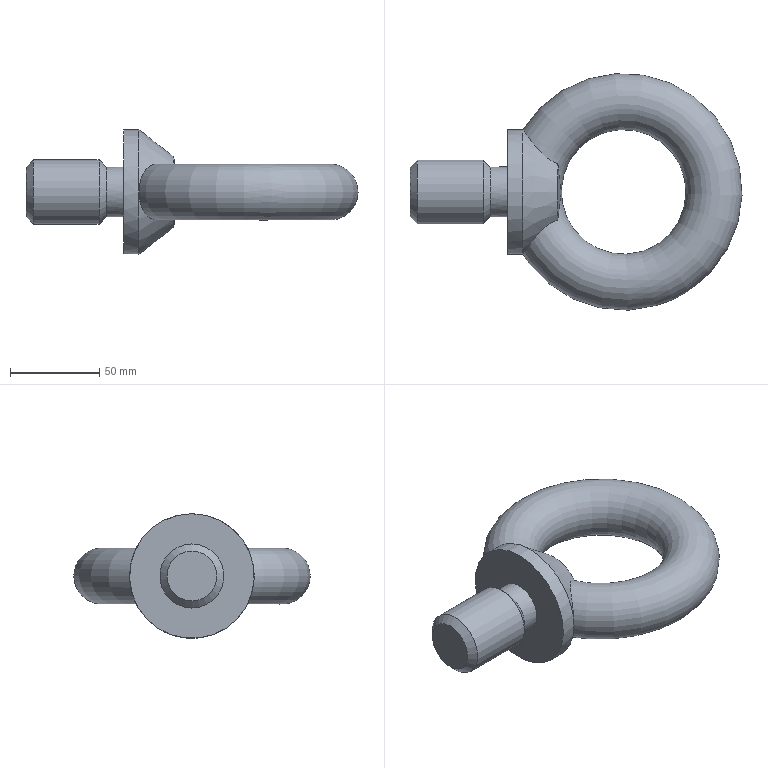Part | NX | features MAIN_BODY 2 | 1 solid | 12 faces | box 186.5 x 133 x 70 mm | volume 340826 mm3 | cone 6 | cylinder 3 | plane 2 | torus 1 | commonest cylinder face diameters 28.02 x1 36 x1 70 x1
STEP:
#1=CARTESIAN_POINT('',(960.853,-771.091,145.));
#2=VERTEX_POINT('',#1);
#3=VERTEX_LOOP('',#2);
#4=FACE_BOUND('',#3,.T.);
#5=CARTESIAN_POINT('',(958.853,-786.916,156.732));
#6=VERTEX_POINT('',#5);
#7=CARTESIAN_POINT('',(958.853,-755.266,156.732));
#8=VERTEX_POINT('',#7);
#9=CARTESIAN_POINT('',(958.853,-786.916,156.732));
#10=CARTESIAN_POINT('',(959.002,-785.546,156.128));
#11=CARTESIAN_POINT('',(959.298,-782.856,154.823));
#12=CARTESIAN_POINT('',(959.669,-779.59,152.997));
#13=CARTESIAN_POINT('',(959.964,-777.027,151.448));
#14=CARTESIAN_POINT('',(960.182,-775.129,150.253));
#15=CARTESIAN_POINT('',(960.359,-773.549,149.234));
#16=CARTESIAN_POINT('',(960.483,-772.275,148.475));
#17=CARTESIAN_POINT('',(960.553,-771.171,148.032));
#18=CARTESIAN_POINT('',(960.496,-770.038,148.397));
#19=CARTESIAN_POINT('',(960.371,-768.751,149.162));
#20=CARTESIAN_POINT('',(960.194,-767.156,150.186));
#21=CARTESIAN_POINT('',(959.974,-765.242,151.394));
#22=CARTESIAN_POINT('',(959.677,-762.658,152.959));
#23=CARTESIAN_POINT('',(959.302,-759.363,154.804));
#24=CARTESIAN_POINT('',(959.003,-756.648,156.122));
#25=CARTESIAN_POINT('',(958.853,-755.266,156.732));
#26=B_SPLINE_CURVE_WITH_KNOTS('',3,(#9,#10,#11,#12,#13,#14,#15,#16,#17,#18,#19,#20,#21,#22,#23,#24,#25),.UNSPECIFIED.,.F.,.F.,(4,1,1,1,1,1,1,1,1,1,1,1,1,1,4),(0.000002027,0.004509,0.009017,0.01127,0.01352,0.01578,0.0169,0.01803,0.01916,0.02028,0.02254,0.02479,0.02705,0.03155,0.03606),.UNSPECIFIED.);
#27=EDGE_CURVE('',#6,#8,#26,.T.);
#28=ORIENTED_EDGE('',*,*,#27,.F.);
#29=CARTESIAN_POINT('',(939.309,-806.091,145.));
#30=VERTEX_POINT('',#29);
#31=CARTESIAN_POINT('',(939.309,-806.091,145.));
#32=CARTESIAN_POINT('',(939.309,-806.091,148.119));
#33=CARTESIAN_POINT('',(940.479,-804.264,154.345));
#34=CARTESIAN_POINT('',(945.008,-797.879,160.146));
#35=CARTESIAN_POINT('',(950.332,-791.897,161.24));
#36=CARTESIAN_POINT('',(955.269,-788.28,159.523));
#37=CARTESIAN_POINT('',(957.716,-787.244,157.784));
#38=CARTESIAN_POINT('',(958.853,-786.916,156.732));
#39=B_SPLINE_CURVE_WITH_KNOTS('',3,(#31,#32,#33,#34,#35,#36,#37,#38),.UNSPECIFIED.,.F.,.F.,(4,1,1,1,1,4),(0.03739,0.04674,0.05608,0.06542,0.07009,0.07477),.UNSPECIFIED.);
#40=EDGE_CURVE('',#30,#6,#39,.T.);
#41=ORIENTED_EDGE('',*,*,#40,.F.);
#42=CARTESIAN_POINT('',(958.853,-786.916,133.268));
#43=VERTEX_POINT('',#42);
#44=CARTESIAN_POINT('',(958.853,-786.916,133.268));
#45=CARTESIAN_POINT('',(957.719,-787.244,132.218));
#46=CARTESIAN_POINT('',(955.279,-788.275,130.484));
#47=CARTESIAN_POINT('',(951.567,-790.987,129.185));
#48=CARTESIAN_POINT('',(948.181,-794.323,129.21));
#49=CARTESIAN_POINT('',(944.234,-798.964,130.833));
#50=CARTESIAN_POINT('',(940.481,-804.265,135.665));
#51=CARTESIAN_POINT('',(939.309,-806.091,141.88));
#52=CARTESIAN_POINT('',(939.309,-806.091,145.));
#53=B_SPLINE_CURVE_WITH_KNOTS('',3,(#44,#45,#46,#47,#48,#49,#50,#51,#52),.UNSPECIFIED.,.F.,.F.,(4,1,1,1,1,1,4),(0.000000275,0.004674,0.009348,0.01402,0.0187,0.02804,0.03739),.UNSPECIFIED.);
#54=EDGE_CURVE('',#43,#30,#53,.T.);
#55=ORIENTED_EDGE('',*,*,#54,.F.);
#56=CARTESIAN_POINT('',(958.853,-755.266,133.268));
#57=VERTEX_POINT('',#56);
#58=CARTESIAN_POINT('',(958.853,-755.266,133.268));
#59=CARTESIAN_POINT('',(959.002,-756.635,133.872));
#60=CARTESIAN_POINT('',(959.298,-759.326,135.177));
#61=CARTESIAN_POINT('',(959.669,-762.592,137.003));
#62=CARTESIAN_POINT('',(959.964,-765.154,138.552));
#63=CARTESIAN_POINT('',(960.182,-767.053,139.747));
#64=CARTESIAN_POINT('',(960.359,-768.633,140.766));
#65=CARTESIAN_POINT('',(960.483,-769.907,141.525));
#66=CARTESIAN_POINT('',(960.553,-771.011,141.968));
#67=CARTESIAN_POINT('',(960.496,-772.143,141.603));
#68=CARTESIAN_POINT('',(960.371,-773.431,140.838));
#69=CARTESIAN_POINT('',(960.194,-775.026,139.814));
#70=CARTESIAN_POINT('',(959.974,-776.94,138.606));
#71=CARTESIAN_POINT('',(959.677,-779.524,137.041));
#72=CARTESIAN_POINT('',(959.302,-782.819,135.196));
#73=CARTESIAN_POINT('',(959.003,-785.534,133.878));
#74=CARTESIAN_POINT('',(958.853,-786.916,133.268));
#75=B_SPLINE_CURVE_WITH_KNOTS('',3,(#58,#59,#60,#61,#62,#63,#64,#65,#66,#67,#68,#69,#70,#71,#72,#73,#74),.UNSPECIFIED.,.F.,.F.,(4,1,1,1,1,1,1,1,1,1,1,1,1,1,4),(0.000002027,0.004509,0.009017,0.01127,0.01352,0.01578,0.0169,0.01803,0.01916,0.02028,0.02254,0.02479,0.02705,0.03155,0.03606),.UNSPECIFIED.);
#76=EDGE_CURVE('',#57,#43,#75,.T.);
#77=ORIENTED_EDGE('',*,*,#76,.F.);
#78=CARTESIAN_POINT('',(939.309,-736.091,145.));
#79=VERTEX_POINT('',#78);
#80=CARTESIAN_POINT('',(939.309,-736.091,145.));
#81=CARTESIAN_POINT('',(939.309,-736.091,141.881));
#82=CARTESIAN_POINT('',(940.479,-737.918,135.655));
#83=CARTESIAN_POINT('',(945.008,-744.303,129.854));
#84=CARTESIAN_POINT('',(950.332,-750.285,128.76));
#85=CARTESIAN_POINT('',(955.269,-753.902,130.477));
#86=CARTESIAN_POINT('',(957.716,-754.937,132.216));
#87=CARTESIAN_POINT('',(958.853,-755.266,133.268));
#88=B_SPLINE_CURVE_WITH_KNOTS('',3,(#80,#81,#82,#83,#84,#85,#86,#87),.UNSPECIFIED.,.F.,.F.,(4,1,1,1,1,4),(0.03739,0.04674,0.05608,0.06542,0.07009,0.07477),.UNSPECIFIED.);
#89=EDGE_CURVE('',#79,#57,#88,.T.);
#90=ORIENTED_EDGE('',*,*,#89,.F.);
#91=CARTESIAN_POINT('',(958.853,-755.266,156.732));
#92=CARTESIAN_POINT('',(957.719,-754.938,157.782));
#93=CARTESIAN_POINT('',(955.279,-753.907,159.516));
#94=CARTESIAN_POINT('',(951.567,-751.195,160.815));
#95=CARTESIAN_POINT('',(948.181,-747.859,160.79));
#96=CARTESIAN_POINT('',(944.234,-743.218,159.167));
#97=CARTESIAN_POINT('',(940.481,-737.917,154.335));
#98=CARTESIAN_POINT('',(939.309,-736.091,148.12));
#99=CARTESIAN_POINT('',(939.309,-736.091,145.));
#100=B_SPLINE_CURVE_WITH_KNOTS('',3,(#91,#92,#93,#94,#95,#96,#97,#98,#99),.UNSPECIFIED.,.F.,.F.,(4,1,1,1,1,1,4),(0.000000275,0.004674,0.009348,0.01402,0.0187,0.02804,0.03739),.UNSPECIFIED.);
#101=EDGE_CURVE('',#8,#79,#100,.T.);
#102=ORIENTED_EDGE('',*,*,#101,.F.);
#103=EDGE_LOOP('',(#28,#41,#55,#77,#90,#102));
#104=FACE_BOUND('',#103,.T.);
#105=CARTESIAN_POINT('',(995.853,-771.091,145.));
#106=DIRECTION('',(0.,0.,-1.));
#107=DIRECTION('',(1.,0.,0.));
#108=AXIS2_PLACEMENT_3D('',#105,#106,#107);
#109=TOROIDAL_SURFACE('',#108,50.75,15.75);
#110=ADVANCED_FACE('',(#4,#104),#109,.T.);
#111=CARTESIAN_POINT('',(930.853,-771.091,180.));
#112=VERTEX_POINT('',#111);
#113=CARTESIAN_POINT('',(930.853,-771.091,145.));
#114=DIRECTION('',(1.,0.,0.));
#115=DIRECTION('',(0.,0.,1.));
#116=AXIS2_PLACEMENT_3D('',#113,#114,#115);
#117=CIRCLE('',#116,35.);
#118=EDGE_CURVE('',#112,#112,#117,.T.);
#119=ORIENTED_EDGE('',*,*,#118,.F.);
#120=EDGE_LOOP('',(#119));
#121=FACE_BOUND('',#120,.T.);
#122=CARTESIAN_POINT('',(930.853,-785.09,144.451));
#123=VERTEX_POINT('',#122);
#124=CARTESIAN_POINT('',(930.853,-757.092,144.451));
#125=VERTEX_POINT('',#124);
#126=CARTESIAN_POINT('',(930.853,-771.091,145.));
#127=DIRECTION('',(1.,0.,0.));
#128=DIRECTION('',(0.,0.,1.));
#129=AXIS2_PLACEMENT_3D('',#126,#127,#128);
#130=CIRCLE('',#129,14.01);
#131=EDGE_CURVE('',#123,#125,#130,.T.);
#132=ORIENTED_EDGE('',*,*,#131,.T.);
#133=CARTESIAN_POINT('',(930.853,-757.092,145.549));
#134=VERTEX_POINT('',#133);
#135=CARTESIAN_POINT('',(930.853,-757.092,144.451));
#136=CARTESIAN_POINT('',(930.853,-757.031,144.817));
#137=CARTESIAN_POINT('',(930.853,-757.031,145.183));
#138=CARTESIAN_POINT('',(930.853,-757.092,145.549));
#139=B_SPLINE_CURVE_WITH_KNOTS('',3,(#135,#136,#137,#138),.UNSPECIFIED.,.F.,.F.,(4,4),(0.,1.),.UNSPECIFIED.);
#140=EDGE_CURVE('',#125,#134,#139,.T.);
#141=ORIENTED_EDGE('',*,*,#140,.T.);
#142=CARTESIAN_POINT('',(930.853,-785.09,145.549));
#143=VERTEX_POINT('',#142);
#144=CARTESIAN_POINT('',(930.853,-771.091,145.));
#145=DIRECTION('',(-1.,0.,0.));
#146=DIRECTION('',(0.,0.,-1.));
#147=AXIS2_PLACEMENT_3D('',#144,#145,#146);
#148=CIRCLE('',#147,14.01);
#149=EDGE_CURVE('',#134,#143,#148,.F.);
#150=ORIENTED_EDGE('',*,*,#149,.T.);
#151=CARTESIAN_POINT('',(930.853,-785.09,145.549));
#152=CARTESIAN_POINT('',(930.853,-785.151,145.183));
#153=CARTESIAN_POINT('',(930.853,-785.151,144.817));
#154=CARTESIAN_POINT('',(930.853,-785.09,144.451));
#155=B_SPLINE_CURVE_WITH_KNOTS('',3,(#151,#152,#153,#154),.UNSPECIFIED.,.F.,.F.,(4,4),(0.,1.),.UNSPECIFIED.);
#156=EDGE_CURVE('',#143,#123,#155,.T.);
#157=ORIENTED_EDGE('',*,*,#156,.T.);
#158=EDGE_LOOP('',(#132,#141,#150,#157));
#159=FACE_BOUND('',#158,.T.);
#160=CARTESIAN_POINT('',(930.853,-771.091,145.));
#161=DIRECTION('',(1.,0.,0.));
#162=DIRECTION('',(0.,0.,1.));
#163=AXIS2_PLACEMENT_3D('',#160,#161,#162);
#164=PLANE('',#163);
#165=ADVANCED_FACE('',(#121,#159),#164,.F.);
#166=CARTESIAN_POINT('',(958.853,-771.091,145.));
#167=DIRECTION('',(1.,0.,0.));
#168=DIRECTION('',(0.,0.,1.));
#169=AXIS2_PLACEMENT_3D('',#166,#167,#168);
#170=CIRCLE('',#169,19.7);
#171=EDGE_CURVE('',#43,#57,#170,.T.);
#172=ORIENTED_EDGE('',*,*,#171,.F.);
#173=ORIENTED_EDGE('',*,*,#54,.T.);
#174=CARTESIAN_POINT('',(939.309,-771.091,145.));
#175=DIRECTION('',(1.,0.,0.));
#176=DIRECTION('',(0.,0.,1.));
#177=AXIS2_PLACEMENT_3D('',#174,#175,#176);
#178=CIRCLE('',#177,35.);
#179=EDGE_CURVE('',#30,#79,#178,.T.);
#180=ORIENTED_EDGE('',*,*,#179,.T.);
#181=ORIENTED_EDGE('',*,*,#89,.T.);
#182=EDGE_LOOP('',(#172,#173,#180,#181));
#183=FACE_BOUND('',#182,.T.);
#184=CARTESIAN_POINT('',(939.309,-771.091,145.));
#185=DIRECTION('',(-1.,0.,0.));
#186=DIRECTION('',(0.,0.,-1.));
#187=AXIS2_PLACEMENT_3D('',#184,#185,#186);
#188=CONICAL_SURFACE('',#187,35.,0.6642);
#189=ADVANCED_FACE('',(#183),#188,.T.);
#190=CARTESIAN_POINT('',(939.309,-771.091,145.));
#191=DIRECTION('',(1.,0.,0.));
#192=DIRECTION('',(0.,0.,1.));
#193=AXIS2_PLACEMENT_3D('',#190,#191,#192);
#194=CIRCLE('',#193,35.);
#195=EDGE_CURVE('',#79,#30,#194,.T.);
#196=ORIENTED_EDGE('',*,*,#195,.T.);
#197=ORIENTED_EDGE('',*,*,#40,.T.);
#198=CARTESIAN_POINT('',(958.853,-771.091,145.));
#199=DIRECTION('',(1.,0.,0.));
#200=DIRECTION('',(0.,0.,1.));
#201=AXIS2_PLACEMENT_3D('',#198,#199,#200);
#202=CIRCLE('',#201,19.7);
#203=EDGE_CURVE('',#8,#6,#202,.T.);
#204=ORIENTED_EDGE('',*,*,#203,.F.);
#205=ORIENTED_EDGE('',*,*,#101,.T.);
#206=EDGE_LOOP('',(#196,#197,#204,#205));
#207=FACE_BOUND('',#206,.T.);
#208=CARTESIAN_POINT('',(939.309,-771.091,145.));
#209=DIRECTION('',(-1.,0.,0.));
#210=DIRECTION('',(0.,0.,-1.));
#211=AXIS2_PLACEMENT_3D('',#208,#209,#210);
#212=CONICAL_SURFACE('',#211,35.,0.6642);
#213=ADVANCED_FACE('',(#207),#212,.T.);
#214=ORIENTED_EDGE('',*,*,#179,.F.);
#215=ORIENTED_EDGE('',*,*,#195,.F.);
#216=EDGE_LOOP('',(#214,#215));
#217=FACE_BOUND('',#216,.T.);
#218=ORIENTED_EDGE('',*,*,#118,.T.);
#219=EDGE_LOOP('',(#218));
#220=FACE_BOUND('',#219,.T.);
#221=CARTESIAN_POINT('',(960.853,-771.091,145.));
#222=DIRECTION('',(1.,0.,0.));
#223=DIRECTION('',(0.,0.,1.));
#224=AXIS2_PLACEMENT_3D('',#221,#222,#223);
#225=CYLINDRICAL_SURFACE('',#224,35.);
#226=ADVANCED_FACE('',(#217,#220),#225,.T.);
#227=CARTESIAN_POINT('',(920.853,-771.091,130.99));
#228=VERTEX_POINT('',#227);
#229=CARTESIAN_POINT('',(920.853,-771.091,145.));
#230=DIRECTION('',(-1.,0.,0.));
#231=DIRECTION('',(0.,0.,-1.));
#232=AXIS2_PLACEMENT_3D('',#229,#230,#231);
#233=CIRCLE('',#232,14.01);
#234=EDGE_CURVE('',#228,#228,#233,.F.);
#235=ORIENTED_EDGE('',*,*,#234,.T.);
#236=EDGE_LOOP('',(#235));
#237=FACE_BOUND('',#236,.T.);
#238=ORIENTED_EDGE('',*,*,#131,.F.);
#239=ORIENTED_EDGE('',*,*,#156,.F.);
#240=ORIENTED_EDGE('',*,*,#149,.F.);
#241=ORIENTED_EDGE('',*,*,#140,.F.);
#242=EDGE_LOOP('',(#238,#239,#240,#241));
#243=FACE_BOUND('',#242,.T.);
#244=CARTESIAN_POINT('',(930.853,-771.091,145.));
#245=DIRECTION('',(-1.,0.,0.));
#246=DIRECTION('',(0.,0.,-1.));
#247=AXIS2_PLACEMENT_3D('',#244,#245,#246);
#248=CYLINDRICAL_SURFACE('',#247,14.01);
#249=ADVANCED_FACE('',(#237,#243),#248,.T.);
#250=CARTESIAN_POINT('',(916.863,-771.091,127.));
#251=VERTEX_POINT('',#250);
#252=CARTESIAN_POINT('',(916.863,-771.091,145.));
#253=DIRECTION('',(-1.,0.,0.));
#254=DIRECTION('',(0.,0.,-1.));
#255=AXIS2_PLACEMENT_3D('',#252,#253,#254);
#256=CIRCLE('',#255,18.);
#257=EDGE_CURVE('',#251,#251,#256,.T.);
#258=ORIENTED_EDGE('',*,*,#257,.T.);
#259=EDGE_LOOP('',(#258));
#260=FACE_BOUND('',#259,.T.);
#261=CARTESIAN_POINT('',(879.843,-771.091,127.));
#262=VERTEX_POINT('',#261);
#263=CARTESIAN_POINT('',(879.843,-771.091,145.));
#264=DIRECTION('',(-1.,0.,0.));
#265=DIRECTION('',(0.,0.,-1.));
#266=AXIS2_PLACEMENT_3D('',#263,#264,#265);
#267=CIRCLE('',#266,18.);
#268=EDGE_CURVE('',#262,#262,#267,.F.);
#269=ORIENTED_EDGE('',*,*,#268,.T.);
#270=EDGE_LOOP('',(#269));
#271=FACE_BOUND('',#270,.T.);
#272=CARTESIAN_POINT('',(875.853,-771.091,145.));
#273=DIRECTION('',(1.,0.,0.));
#274=DIRECTION('',(0.,0.,1.));
#275=AXIS2_PLACEMENT_3D('',#272,#273,#274);
#276=CYLINDRICAL_SURFACE('',#275,18.);
#277=ADVANCED_FACE('',(#260,#271),#276,.T.);
#278=CARTESIAN_POINT('',(875.853,-771.091,130.99));
#279=VERTEX_POINT('',#278);
#280=CARTESIAN_POINT('',(875.853,-771.091,145.));
#281=DIRECTION('',(-1.,0.,0.));
#282=DIRECTION('',(0.,0.,-1.));
#283=AXIS2_PLACEMENT_3D('',#280,#281,#282);
#284=CIRCLE('',#283,14.01);
#285=EDGE_CURVE('',#279,#279,#284,.T.);
#286=ORIENTED_EDGE('',*,*,#285,.T.);
#287=EDGE_LOOP('',(#286));
#288=FACE_BOUND('',#287,.T.);
#289=CARTESIAN_POINT('',(875.853,-771.091,145.));
#290=DIRECTION('',(-1.,0.,0.));
#291=DIRECTION('',(0.,0.,-1.));
#292=AXIS2_PLACEMENT_3D('',#289,#290,#291);
#293=PLANE('',#292);
#294=ADVANCED_FACE('',(#288),#293,.T.);
#295=ORIENTED_EDGE('',*,*,#268,.F.);
#296=EDGE_LOOP('',(#295));
#297=FACE_BOUND('',#296,.T.);
#298=ORIENTED_EDGE('',*,*,#285,.F.);
#299=EDGE_LOOP('',(#298));
#300=FACE_BOUND('',#299,.T.);
#301=CARTESIAN_POINT('',(875.853,-771.091,145.));
#302=DIRECTION('',(1.,0.,0.));
#303=DIRECTION('',(0.,0.,1.));
#304=AXIS2_PLACEMENT_3D('',#301,#302,#303);
#305=CONICAL_SURFACE('',#304,14.01,0.7854);
#306=ADVANCED_FACE('',(#297,#300),#305,.T.);
#307=ORIENTED_EDGE('',*,*,#234,.F.);
#308=EDGE_LOOP('',(#307));
#309=FACE_BOUND('',#308,.T.);
#310=ORIENTED_EDGE('',*,*,#257,.F.);
#311=EDGE_LOOP('',(#310));
#312=FACE_BOUND('',#311,.T.);
#313=CARTESIAN_POINT('',(916.863,-771.091,145.));
#314=DIRECTION('',(-1.,0.,0.));
#315=DIRECTION('',(0.,0.,-1.));
#316=AXIS2_PLACEMENT_3D('',#313,#314,#315);
#317=CONICAL_SURFACE('',#316,18.,0.7854);
#318=ADVANCED_FACE('',(#309,#312),#317,.T.);
#319=ORIENTED_EDGE('',*,*,#171,.T.);
#320=ORIENTED_EDGE('',*,*,#76,.T.);
#321=EDGE_LOOP('',(#319,#320));
#322=FACE_BOUND('',#321,.T.);
#323=CARTESIAN_POINT('',(958.853,-771.091,145.));
#324=DIRECTION('',(-1.,0.,0.));
#325=DIRECTION('',(0.,0.,-1.));
#326=AXIS2_PLACEMENT_3D('',#323,#324,#325);
#327=CONICAL_SURFACE('',#326,19.7,1.47);
#328=ADVANCED_FACE('',(#322),#327,.T.);
#329=ORIENTED_EDGE('',*,*,#203,.T.);
#330=ORIENTED_EDGE('',*,*,#27,.T.);
#331=EDGE_LOOP('',(#329,#330));
#332=FACE_BOUND('',#331,.T.);
#333=CARTESIAN_POINT('',(958.853,-771.091,145.));
#334=DIRECTION('',(-1.,0.,0.));
#335=DIRECTION('',(0.,0.,-1.));
#336=AXIS2_PLACEMENT_3D('',#333,#334,#335);
#337=CONICAL_SURFACE('',#336,19.7,1.47);
#338=ADVANCED_FACE('',(#332),#337,.T.);
#339=CLOSED_SHELL('',(#110,#165,#189,#213,#226,#249,#277,#294,#306,#318,#328,#338));
#340=MANIFOLD_SOLID_BREP('',#339);
#341=(LENGTH_UNIT()NAMED_UNIT(*)SI_UNIT(.MILLI.,.METRE.));
#342=UNCERTAINTY_MEASURE_WITH_UNIT(LENGTH_MEASURE(0.1034),#341,'','');
#343=(NAMED_UNIT(*)PLANE_ANGLE_UNIT()SI_UNIT($,.RADIAN.));
#344=(NAMED_UNIT(*)SI_UNIT($,.STERADIAN.)SOLID_ANGLE_UNIT());
#345=(GEOMETRIC_REPRESENTATION_CONTEXT(3)GLOBAL_UNCERTAINTY_ASSIGNED_CONTEXT((#342))GLOBAL_UNIT_ASSIGNED_CONTEXT((#341,#343,#344))REPRESENTATION_CONTEXT('',''));
#346=ADVANCED_BREP_SHAPE_REPRESENTATION('',(#340),#345);